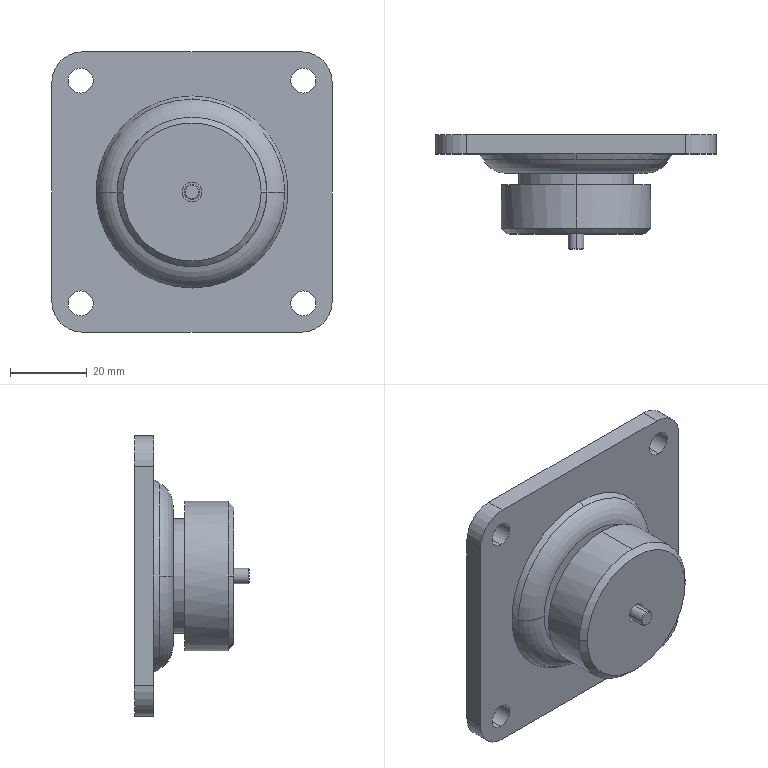Part | STEP file | HJHI_CGR51-60-U-003 | 1 solid | 72 faces | box 73 x 29.8 x 73 mm | volume 47628 mm3 | plane 34 | cylinder 26 | cone 10 | torus 2 | commonest cylinder face diameters 6.5 x8 16 x4 4 x2 5.2 x2 10 x2 12 x2